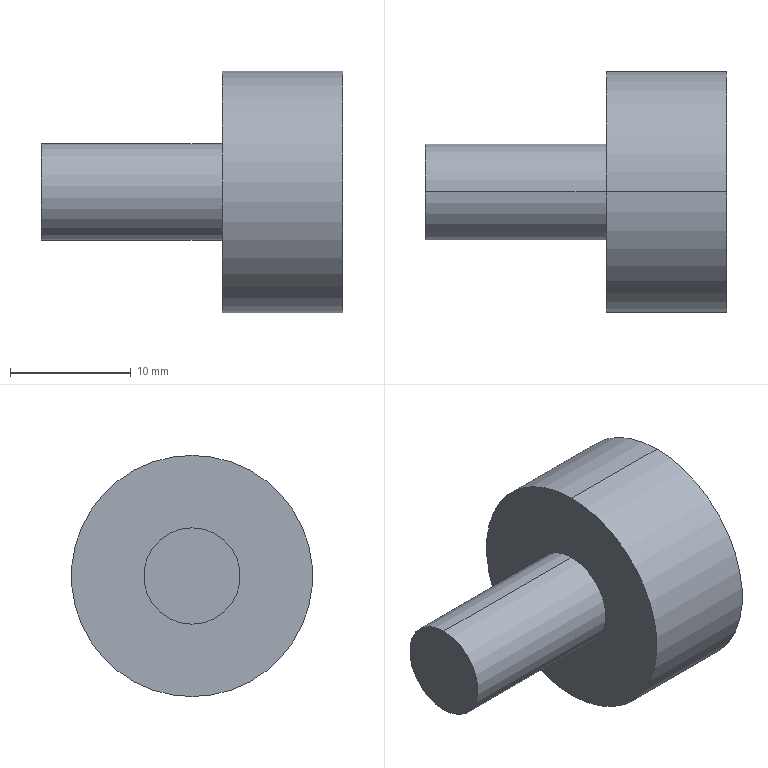Part | SolidWorks | features Extrusion 1, HoleWzd 1, ICE 1 | 1 solid | 11 faces | box 25 x 20 x 20 mm | volume 3580 mm3 | cylinder 6 | plane 3 | cone 2 | commonest cylinder face diameters 6.8 x2 8 x2 20 x2
STEP:
#1=CARTESIAN_POINT('',(2.,0.,3.4));
#2=VERTEX_POINT('',#1);
#3=CARTESIAN_POINT('',(2.,0.,-3.4));
#4=VERTEX_POINT('',#3);
#5=CARTESIAN_POINT('',(2.,0.,0.));
#6=DIRECTION('',(1.,0.,0.));
#7=DIRECTION('',(0.,0.,-1.));
#8=AXIS2_PLACEMENT_3D('',#5,#6,#7);
#9=CIRCLE('',#8,3.4);
#10=EDGE_CURVE('',#2,#4,#9,.T.);
#11=ORIENTED_EDGE('',*,*,#10,.F.);
#12=CARTESIAN_POINT('',(10.,0.,3.4));
#13=VERTEX_POINT('',#12);
#14=CARTESIAN_POINT('',(10.,0.,3.4));
#15=DIRECTION('',(1.,0.,0.));
#16=VECTOR('',#15,1000.);
#17=LINE('',#14,#16);
#18=EDGE_CURVE('',#2,#13,#17,.T.);
#19=ORIENTED_EDGE('',*,*,#18,.T.);
#20=CARTESIAN_POINT('',(10.,0.,-3.4));
#21=VERTEX_POINT('',#20);
#22=CARTESIAN_POINT('',(10.,0.,0.));
#23=DIRECTION('',(1.,0.,0.));
#24=DIRECTION('',(0.,0.,-1.));
#25=AXIS2_PLACEMENT_3D('',#22,#23,#24);
#26=CIRCLE('',#25,3.4);
#27=EDGE_CURVE('',#13,#21,#26,.T.);
#28=ORIENTED_EDGE('',*,*,#27,.T.);
#29=CARTESIAN_POINT('',(10.,0.,-3.4));
#30=DIRECTION('',(1.,0.,0.));
#31=VECTOR('',#30,1000.);
#32=LINE('',#29,#31);
#33=EDGE_CURVE('',#4,#21,#32,.T.);
#34=ORIENTED_EDGE('',*,*,#33,.F.);
#35=EDGE_LOOP('',(#11,#19,#28,#34));
#36=FACE_OUTER_BOUND('',#35,.T.);
#37=CARTESIAN_POINT('',(10.,0.,0.));
#38=DIRECTION('',(1.,0.,0.));
#39=DIRECTION('',(0.,0.,-1.));
#40=AXIS2_PLACEMENT_3D('',#37,#38,#39);
#41=CYLINDRICAL_SURFACE('',#40,3.4);
#42=ADVANCED_FACE('',(#36),#41,.F.);
#43=CARTESIAN_POINT('',(-0.04293,0.,0.));
#44=VERTEX_POINT('',#43);
#45=CARTESIAN_POINT('',(2.,0.,-3.4));
#46=DIRECTION('',(0.515,0.,-0.8572));
#47=VECTOR('',#46,1000.);
#48=LINE('',#45,#47);
#49=EDGE_CURVE('',#44,#4,#48,.T.);
#50=ORIENTED_EDGE('',*,*,#49,.F.);
#51=CARTESIAN_POINT('',(2.,0.,3.4));
#52=DIRECTION('',(0.515,0.,0.8572));
#53=VECTOR('',#52,1000.);
#54=LINE('',#51,#53);
#55=EDGE_CURVE('',#44,#2,#54,.T.);
#56=ORIENTED_EDGE('',*,*,#55,.T.);
#57=ORIENTED_EDGE('',*,*,#10,.T.);
#58=EDGE_LOOP('',(#50,#56,#57));
#59=FACE_OUTER_BOUND('',#58,.T.);
#60=CARTESIAN_POINT('',(2.,0.,0.));
#61=DIRECTION('',(1.,0.,0.));
#62=DIRECTION('',(0.,0.,-1.));
#63=AXIS2_PLACEMENT_3D('',#60,#61,#62);
#64=CONICAL_SURFACE('',#63,3.4,1.03);
#65=ADVANCED_FACE('',(#59),#64,.F.);
#66=CARTESIAN_POINT('',(-15.,0.,4.));
#67=VERTEX_POINT('',#66);
#68=CARTESIAN_POINT('',(-15.,0.,-4.));
#69=VERTEX_POINT('',#68);
#70=CARTESIAN_POINT('',(-15.,0.,0.));
#71=DIRECTION('',(-1.,0.,0.));
#72=DIRECTION('',(0.,0.,1.));
#73=AXIS2_PLACEMENT_3D('',#70,#71,#72);
#74=CIRCLE('',#73,4.);
#75=EDGE_CURVE('',#67,#69,#74,.T.);
#76=ORIENTED_EDGE('',*,*,#75,.F.);
#77=CARTESIAN_POINT('',(0.,0.,4.));
#78=VERTEX_POINT('',#77);
#79=CARTESIAN_POINT('',(-15.,0.,4.));
#80=DIRECTION('',(1.,0.,0.));
#81=VECTOR('',#80,1000.);
#82=LINE('',#79,#81);
#83=EDGE_CURVE('',#67,#78,#82,.T.);
#84=ORIENTED_EDGE('',*,*,#83,.T.);
#85=CARTESIAN_POINT('',(0.,0.,-4.));
#86=VERTEX_POINT('',#85);
#87=CARTESIAN_POINT('',(0.,0.,0.));
#88=DIRECTION('',(-1.,0.,0.));
#89=DIRECTION('',(0.,0.,1.));
#90=AXIS2_PLACEMENT_3D('',#87,#88,#89);
#91=CIRCLE('',#90,4.);
#92=EDGE_CURVE('',#78,#86,#91,.T.);
#93=ORIENTED_EDGE('',*,*,#92,.T.);
#94=CARTESIAN_POINT('',(-15.,0.,-4.));
#95=DIRECTION('',(1.,0.,0.));
#96=VECTOR('',#95,1000.);
#97=LINE('',#94,#96);
#98=EDGE_CURVE('',#69,#86,#97,.T.);
#99=ORIENTED_EDGE('',*,*,#98,.F.);
#100=EDGE_LOOP('',(#76,#84,#93,#99));
#101=FACE_OUTER_BOUND('',#100,.T.);
#102=CARTESIAN_POINT('',(-15.,0.,0.));
#103=DIRECTION('',(1.,0.,0.));
#104=DIRECTION('',(0.,0.,-1.));
#105=AXIS2_PLACEMENT_3D('',#102,#103,#104);
#106=CYLINDRICAL_SURFACE('',#105,4.);
#107=ADVANCED_FACE('',(#101),#106,.T.);
#108=CARTESIAN_POINT('',(10.,0.,-10.));
#109=VERTEX_POINT('',#108);
#110=CARTESIAN_POINT('',(10.,0.,10.));
#111=VERTEX_POINT('',#110);
#112=CARTESIAN_POINT('',(10.,0.,0.));
#113=DIRECTION('',(1.,0.,0.));
#114=DIRECTION('',(0.,0.,-1.));
#115=AXIS2_PLACEMENT_3D('',#112,#113,#114);
#116=CIRCLE('',#115,10.);
#117=EDGE_CURVE('',#109,#111,#116,.T.);
#118=ORIENTED_EDGE('',*,*,#117,.F.);
#119=CARTESIAN_POINT('',(0.,0.,-10.));
#120=VERTEX_POINT('',#119);
#121=CARTESIAN_POINT('',(10.,0.,-10.));
#122=DIRECTION('',(-1.,0.,0.));
#123=VECTOR('',#122,1000.);
#124=LINE('',#121,#123);
#125=EDGE_CURVE('',#109,#120,#124,.T.);
#126=ORIENTED_EDGE('',*,*,#125,.T.);
#127=CARTESIAN_POINT('',(0.,0.,10.));
#128=VERTEX_POINT('',#127);
#129=CARTESIAN_POINT('',(0.,0.,0.));
#130=DIRECTION('',(1.,0.,0.));
#131=DIRECTION('',(0.,0.,-1.));
#132=AXIS2_PLACEMENT_3D('',#129,#130,#131);
#133=CIRCLE('',#132,10.);
#134=EDGE_CURVE('',#120,#128,#133,.T.);
#135=ORIENTED_EDGE('',*,*,#134,.T.);
#136=CARTESIAN_POINT('',(10.,0.,10.));
#137=DIRECTION('',(-1.,0.,0.));
#138=VECTOR('',#137,1000.);
#139=LINE('',#136,#138);
#140=EDGE_CURVE('',#111,#128,#139,.T.);
#141=ORIENTED_EDGE('',*,*,#140,.F.);
#142=EDGE_LOOP('',(#118,#126,#135,#141));
#143=FACE_OUTER_BOUND('',#142,.T.);
#144=CARTESIAN_POINT('',(10.,0.,0.));
#145=DIRECTION('',(-1.,0.,0.));
#146=DIRECTION('',(0.,0.,1.));
#147=AXIS2_PLACEMENT_3D('',#144,#145,#146);
#148=CYLINDRICAL_SURFACE('',#147,10.);
#149=ADVANCED_FACE('',(#143),#148,.T.);
#150=ORIENTED_EDGE('',*,*,#125,.F.);
#151=CARTESIAN_POINT('',(10.,0.,0.));
#152=DIRECTION('',(1.,0.,0.));
#153=DIRECTION('',(0.,0.,-1.));
#154=AXIS2_PLACEMENT_3D('',#151,#152,#153);
#155=CIRCLE('',#154,10.);
#156=EDGE_CURVE('',#111,#109,#155,.T.);
#157=ORIENTED_EDGE('',*,*,#156,.F.);
#158=ORIENTED_EDGE('',*,*,#140,.T.);
#159=CARTESIAN_POINT('',(0.,0.,0.));
#160=DIRECTION('',(1.,0.,0.));
#161=DIRECTION('',(0.,0.,-1.));
#162=AXIS2_PLACEMENT_3D('',#159,#160,#161);
#163=CIRCLE('',#162,10.);
#164=EDGE_CURVE('',#128,#120,#163,.T.);
#165=ORIENTED_EDGE('',*,*,#164,.T.);
#166=EDGE_LOOP('',(#150,#157,#158,#165));
#167=FACE_OUTER_BOUND('',#166,.T.);
#168=CARTESIAN_POINT('',(10.,0.,0.));
#169=DIRECTION('',(-1.,0.,0.));
#170=DIRECTION('',(0.,0.,1.));
#171=AXIS2_PLACEMENT_3D('',#168,#169,#170);
#172=CYLINDRICAL_SURFACE('',#171,10.);
#173=ADVANCED_FACE('',(#167),#172,.T.);
#174=CARTESIAN_POINT('',(10.,0.,0.));
#175=DIRECTION('',(1.,0.,0.));
#176=DIRECTION('',(0.,0.,-1.));
#177=AXIS2_PLACEMENT_3D('',#174,#175,#176);
#178=CIRCLE('',#177,3.4);
#179=EDGE_CURVE('',#21,#13,#178,.T.);
#180=ORIENTED_EDGE('',*,*,#179,.F.);
#181=ORIENTED_EDGE('',*,*,#27,.F.);
#182=EDGE_LOOP('',(#180,#181));
#183=FACE_BOUND('',#182,.T.);
#184=ORIENTED_EDGE('',*,*,#156,.T.);
#185=ORIENTED_EDGE('',*,*,#117,.T.);
#186=EDGE_LOOP('',(#184,#185));
#187=FACE_OUTER_BOUND('',#186,.T.);
#188=CARTESIAN_POINT('',(10.,0.,0.));
#189=DIRECTION('',(1.,0.,0.));
#190=DIRECTION('',(0.,0.,-1.));
#191=AXIS2_PLACEMENT_3D('',#188,#189,#190);
#192=PLANE('',#191);
#193=ADVANCED_FACE('',(#183,#187),#192,.T.);
#194=CARTESIAN_POINT('',(0.,0.,0.));
#195=DIRECTION('',(-1.,0.,0.));
#196=DIRECTION('',(0.,0.,1.));
#197=AXIS2_PLACEMENT_3D('',#194,#195,#196);
#198=CIRCLE('',#197,4.);
#199=EDGE_CURVE('',#86,#78,#198,.T.);
#200=ORIENTED_EDGE('',*,*,#199,.F.);
#201=ORIENTED_EDGE('',*,*,#92,.F.);
#202=EDGE_LOOP('',(#200,#201));
#203=FACE_BOUND('',#202,.T.);
#204=ORIENTED_EDGE('',*,*,#164,.F.);
#205=ORIENTED_EDGE('',*,*,#134,.F.);
#206=EDGE_LOOP('',(#204,#205));
#207=FACE_OUTER_BOUND('',#206,.T.);
#208=CARTESIAN_POINT('',(0.,0.,0.));
#209=DIRECTION('',(1.,0.,0.));
#210=DIRECTION('',(0.,0.,-1.));
#211=AXIS2_PLACEMENT_3D('',#208,#209,#210);
#212=PLANE('',#211);
#213=ADVANCED_FACE('',(#203,#207),#212,.F.);
#214=ORIENTED_EDGE('',*,*,#83,.F.);
#215=CARTESIAN_POINT('',(-15.,0.,0.));
#216=DIRECTION('',(-1.,0.,0.));
#217=DIRECTION('',(0.,0.,1.));
#218=AXIS2_PLACEMENT_3D('',#215,#216,#217);
#219=CIRCLE('',#218,4.);
#220=EDGE_CURVE('',#69,#67,#219,.T.);
#221=ORIENTED_EDGE('',*,*,#220,.F.);
#222=ORIENTED_EDGE('',*,*,#98,.T.);
#223=ORIENTED_EDGE('',*,*,#199,.T.);
#224=EDGE_LOOP('',(#214,#221,#222,#223));
#225=FACE_OUTER_BOUND('',#224,.T.);
#226=CARTESIAN_POINT('',(-15.,0.,0.));
#227=DIRECTION('',(1.,0.,0.));
#228=DIRECTION('',(0.,0.,-1.));
#229=AXIS2_PLACEMENT_3D('',#226,#227,#228);
#230=CYLINDRICAL_SURFACE('',#229,4.);
#231=ADVANCED_FACE('',(#225),#230,.T.);
#232=ORIENTED_EDGE('',*,*,#220,.T.);
#233=ORIENTED_EDGE('',*,*,#75,.T.);
#234=EDGE_LOOP('',(#232,#233));
#235=FACE_OUTER_BOUND('',#234,.T.);
#236=CARTESIAN_POINT('',(-15.,0.,0.));
#237=DIRECTION('',(-1.,0.,0.));
#238=DIRECTION('',(0.,0.,1.));
#239=AXIS2_PLACEMENT_3D('',#236,#237,#238);
#240=PLANE('',#239);
#241=ADVANCED_FACE('',(#235),#240,.T.);
#242=ORIENTED_EDGE('',*,*,#55,.F.);
#243=ORIENTED_EDGE('',*,*,#49,.T.);
#244=CARTESIAN_POINT('',(2.,0.,0.));
#245=DIRECTION('',(1.,0.,0.));
#246=DIRECTION('',(0.,0.,-1.));
#247=AXIS2_PLACEMENT_3D('',#244,#245,#246);
#248=CIRCLE('',#247,3.4);
#249=EDGE_CURVE('',#4,#2,#248,.T.);
#250=ORIENTED_EDGE('',*,*,#249,.T.);
#251=EDGE_LOOP('',(#242,#243,#250));
#252=FACE_OUTER_BOUND('',#251,.T.);
#253=CARTESIAN_POINT('',(2.,0.,0.));
#254=DIRECTION('',(1.,0.,0.));
#255=DIRECTION('',(0.,0.,-1.));
#256=AXIS2_PLACEMENT_3D('',#253,#254,#255);
#257=CONICAL_SURFACE('',#256,3.4,1.03);
#258=ADVANCED_FACE('',(#252),#257,.F.);
#259=ORIENTED_EDGE('',*,*,#18,.F.);
#260=ORIENTED_EDGE('',*,*,#249,.F.);
#261=ORIENTED_EDGE('',*,*,#33,.T.);
#262=ORIENTED_EDGE('',*,*,#179,.T.);
#263=EDGE_LOOP('',(#259,#260,#261,#262));
#264=FACE_OUTER_BOUND('',#263,.T.);
#265=CARTESIAN_POINT('',(10.,0.,0.));
#266=DIRECTION('',(1.,0.,0.));
#267=DIRECTION('',(0.,0.,-1.));
#268=AXIS2_PLACEMENT_3D('',#265,#266,#267);
#269=CYLINDRICAL_SURFACE('',#268,3.4);
#270=ADVANCED_FACE('',(#264),#269,.F.);
#271=CLOSED_SHELL('',(#42,#65,#107,#149,#173,#193,#213,#231,#241,#258,#270));
#272=MANIFOLD_SOLID_BREP('',#271);
#273=CARTESIAN_POINT('',(0.,0.,0.));
#274=DIRECTION('',(0.,0.,1.));
#275=DIRECTION('',(1.,0.,0.));
#276=AXIS2_PLACEMENT_3D('',#273,#274,#275);
#277=(LENGTH_UNIT()NAMED_UNIT(*)SI_UNIT(.MILLI.,.METRE.));
#278=UNCERTAINTY_MEASURE_WITH_UNIT(LENGTH_MEASURE(0.00001),#277,'','');
#279=(NAMED_UNIT(*)PLANE_ANGLE_UNIT()SI_UNIT($,.RADIAN.));
#280=(NAMED_UNIT(*)SI_UNIT($,.STERADIAN.)SOLID_ANGLE_UNIT());
#281=(GEOMETRIC_REPRESENTATION_CONTEXT(3)GLOBAL_UNCERTAINTY_ASSIGNED_CONTEXT((#278))GLOBAL_UNIT_ASSIGNED_CONTEXT((#277,#279,#280))REPRESENTATION_CONTEXT('',''));
#282=ADVANCED_BREP_SHAPE_REPRESENTATION('',(#272,#276),#281);